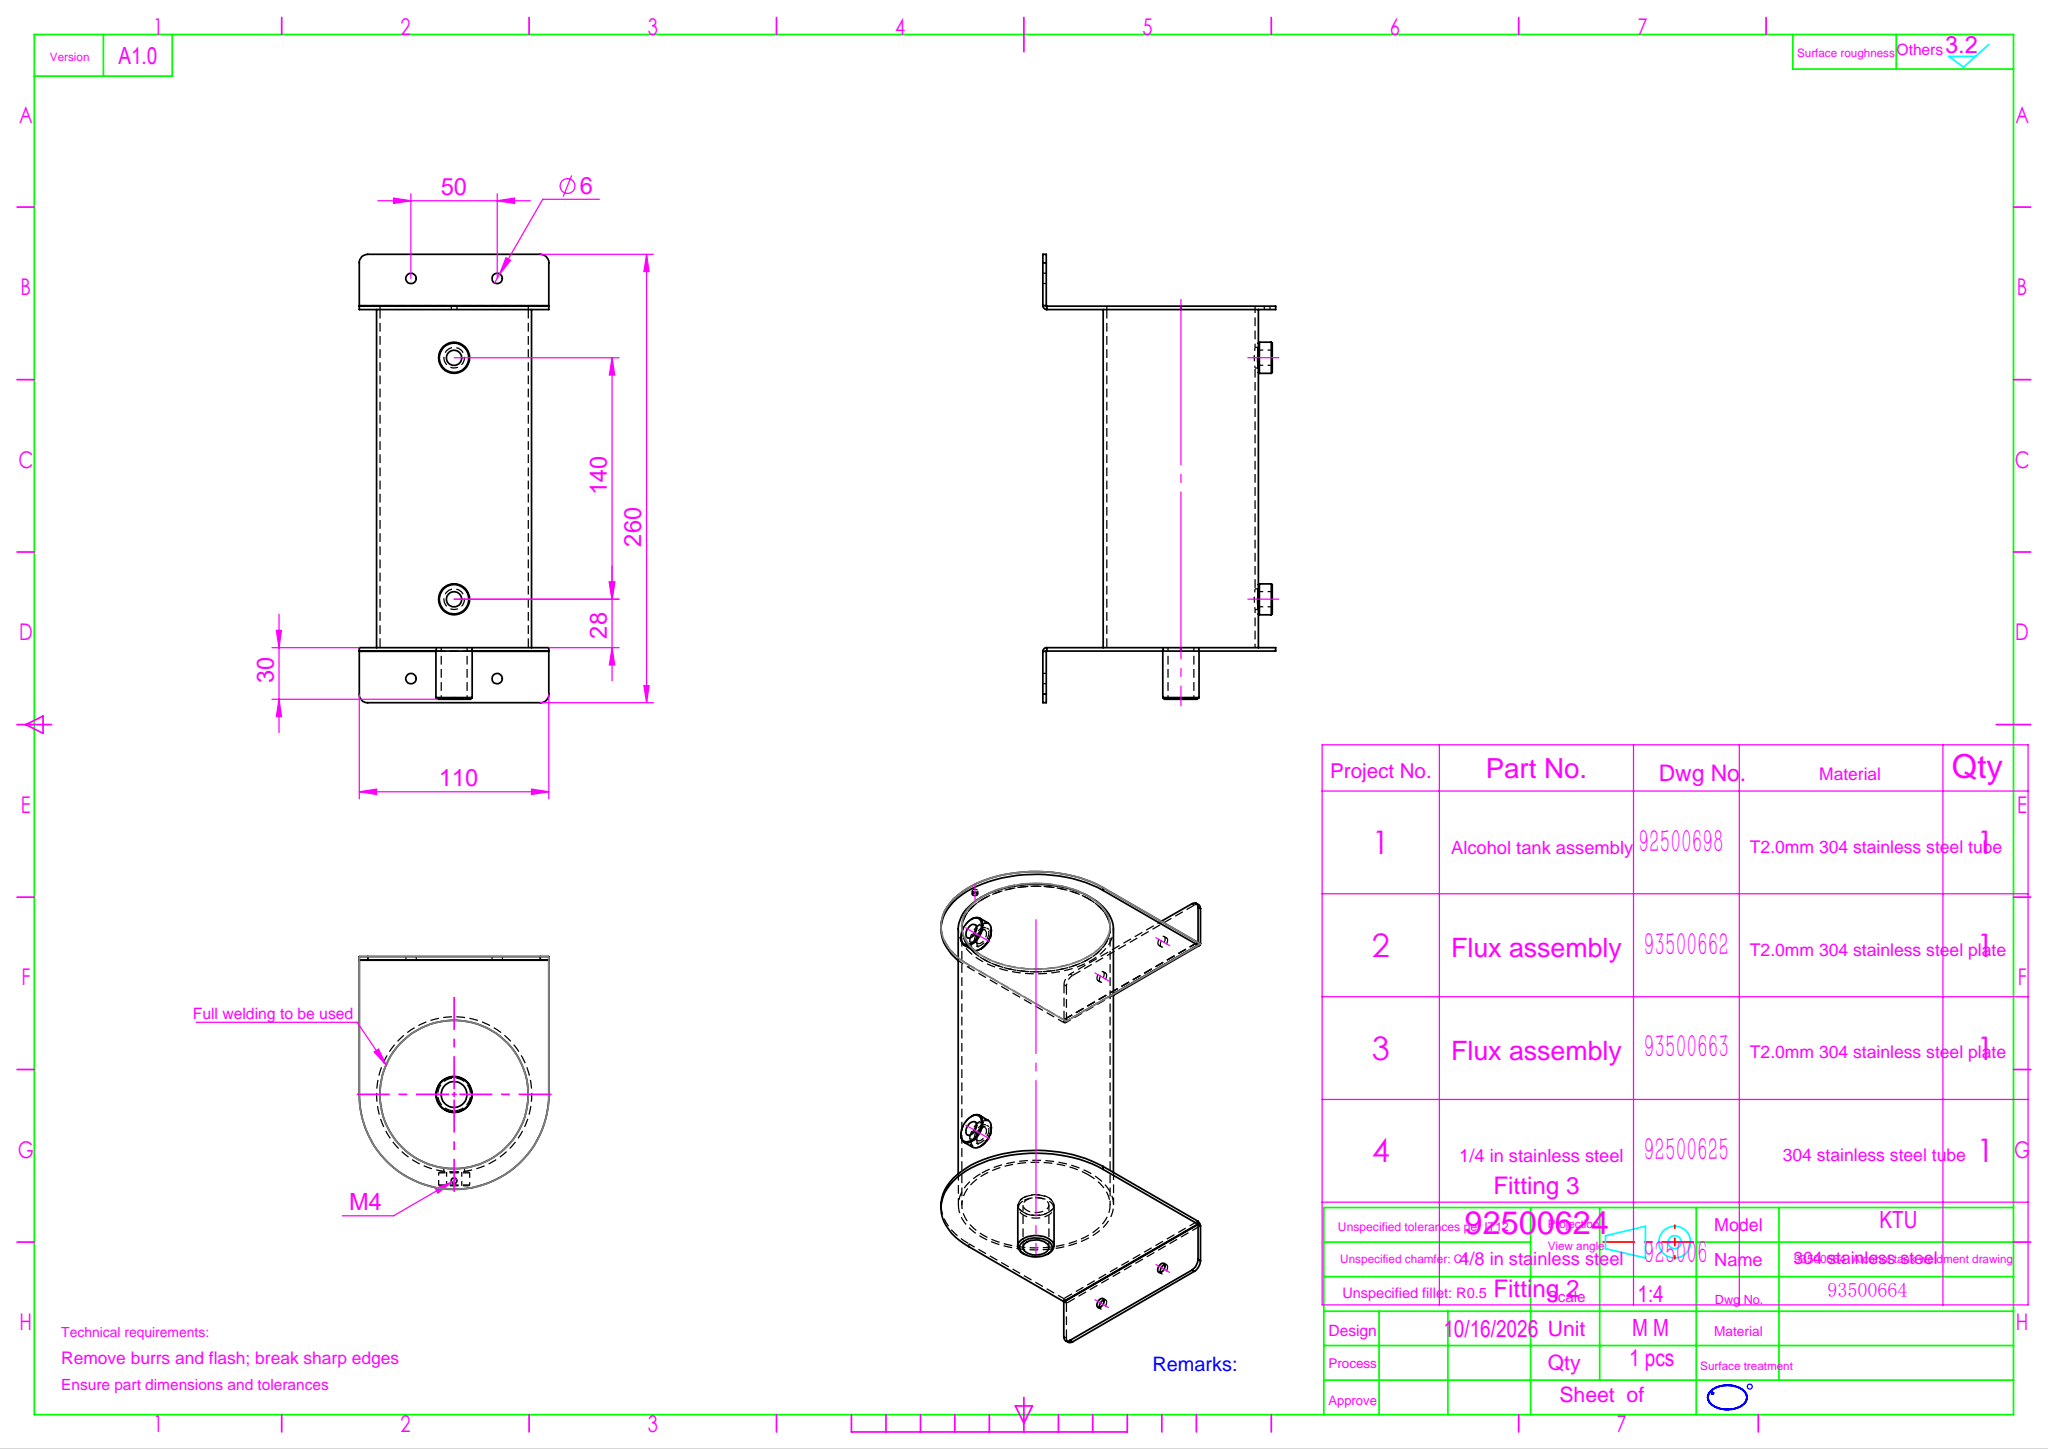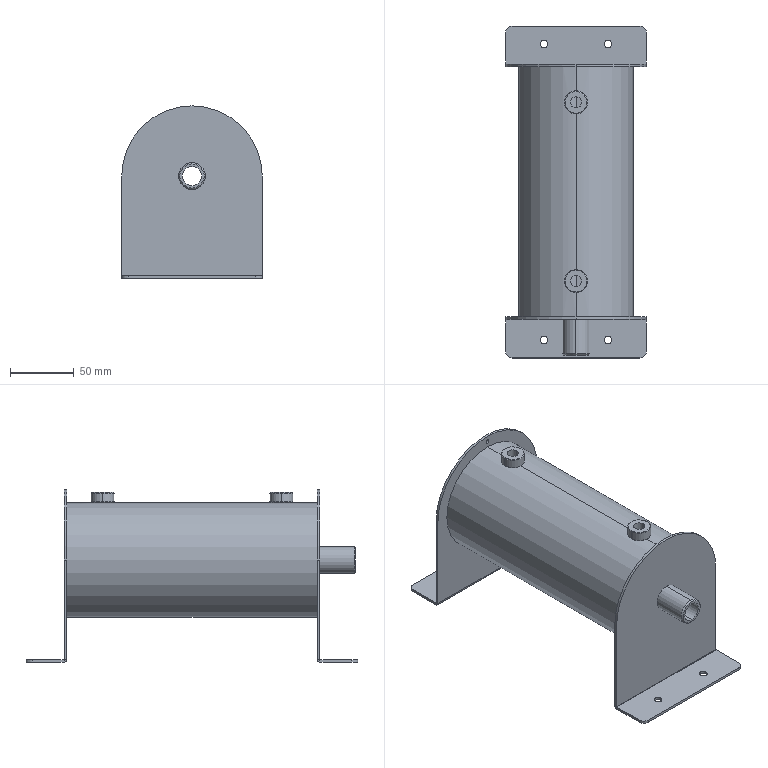Part | SolidWorks | features CompositeCurve 1 | 6 solids | 86 faces | box 110 x 260 x 135 mm | volume 170663 mm3 | cylinder 46 | plane 30 | cone 10 | commonest cylinder face diameters 6 x8 8.8 x4 10 x4 12 x4 18 x4 86 x4